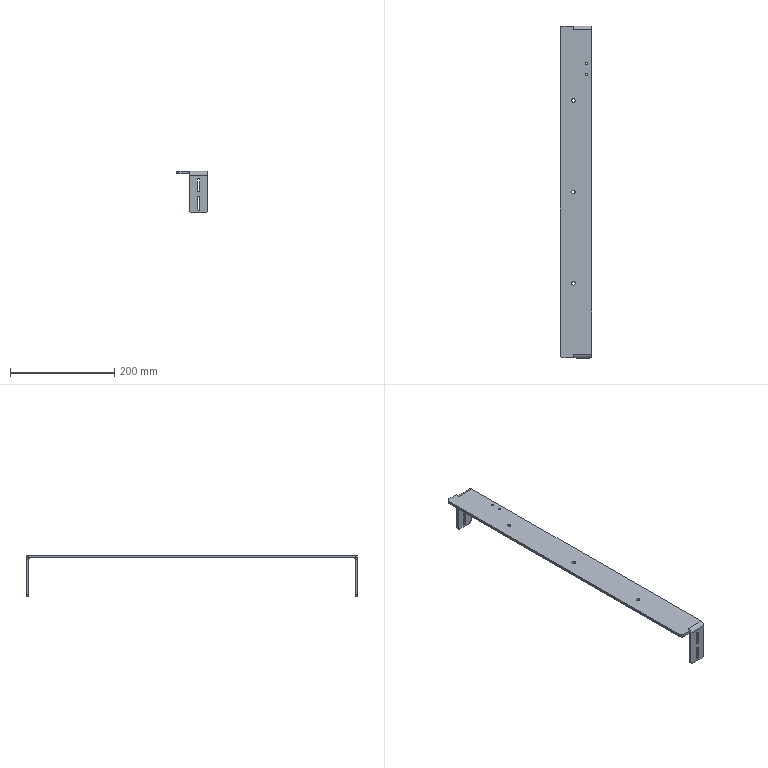Part | STEP file | 1 solid | 68 faces | box 60 x 636 x 80 mm | volume 212766 mm3 | cylinder 32 | plane 30 | cone 6 | commonest cylinder face diameters 5.5 x12 6.8 x6 10 x6 4.2 x4 5 x2 15 x2